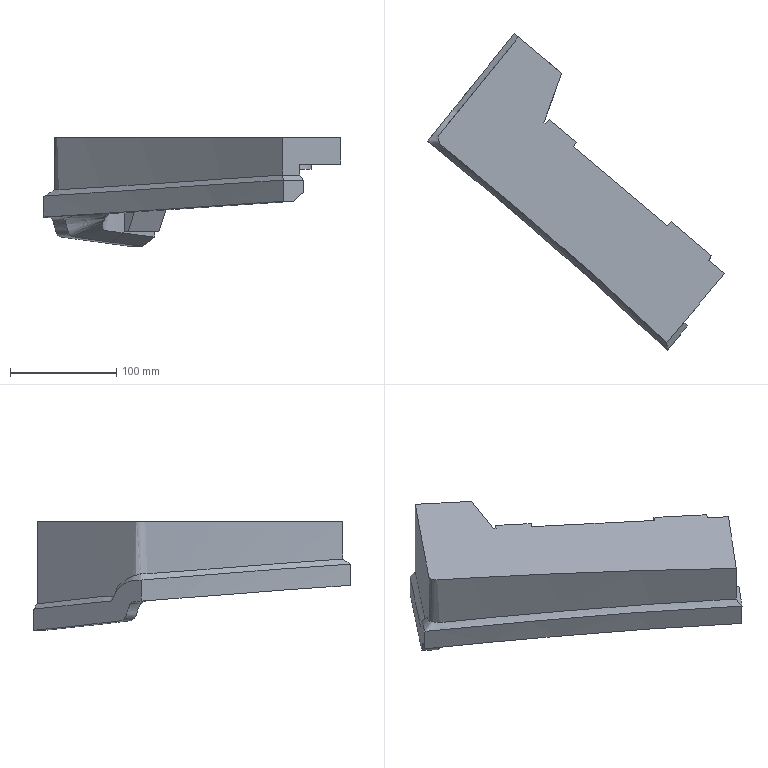Part | NX | features solid 2 | 1 solid | 35 faces | box 280.196 x 298.557 x 102.669 mm | volume 1274307 mm3 | plane 24 | spline 7 | cylinder 4 | commonest cylinder face diameters 30 x4